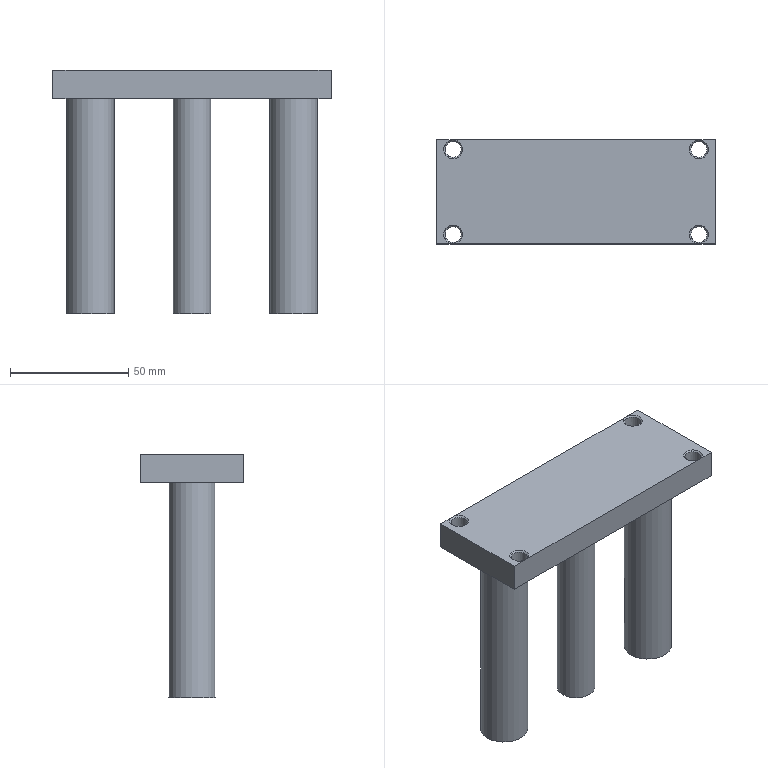Part | STEP file | Tube necking machine_id334_x_t | 1 solid | 24 faces | box 118 x 44 x 103 mm | volume 136002 mm3 | plane 9 | cone 8 | cylinder 7 | commonest cylinder face diameters 6.8 x4 20 x2 16 x1